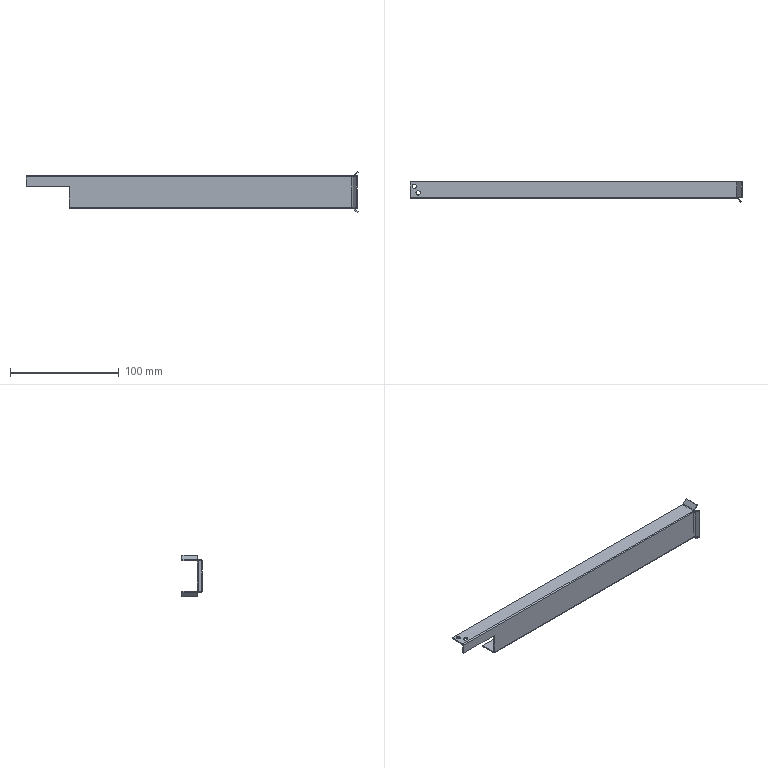Part | NX | 1 solid | 39 faces | box 305.707 x 18.464 x 38.21 mm | volume 16264 mm3 | plane 22 | cylinder 15 | torus 2 | commonest cylinder face diameters 4 x6 2 x4 6 x4 2.56 x1
STEP:
#1=CARTESIAN_POINT('',(150.133,-6.501,-15.));
#2=VERTEX_POINT('',#1);
#3=CARTESIAN_POINT('',(150.133,7.5,-15.));
#4=VERTEX_POINT('',#3);
#5=CARTESIAN_POINT('',(150.133,7.5,-15.));
#6=DIRECTION('',(0.,1.,0.));
#7=VECTOR('',#6,1000.);
#8=LINE('',#5,#7);
#9=EDGE_CURVE('',#2,#4,#8,.T.);
#10=ORIENTED_EDGE('',*,*,#9,.F.);
#11=CARTESIAN_POINT('',(150.,-6.5,-15.));
#12=VERTEX_POINT('',#11);
#13=CARTESIAN_POINT('',(150.,-9.5,-15.));
#14=DIRECTION('',(0.,0.,-1.));
#15=DIRECTION('',(0.,1.,0.));
#16=AXIS2_PLACEMENT_3D('',#13,#14,#15);
#17=CIRCLE('',#16,3.);
#18=EDGE_CURVE('',#12,#2,#17,.T.);
#19=ORIENTED_EDGE('',*,*,#18,.F.);
#20=CARTESIAN_POINT('',(-110.,-6.5,-15.));
#21=VERTEX_POINT('',#20);
#22=CARTESIAN_POINT('',(150.722,-6.5,-15.));
#23=DIRECTION('',(-1.,0.,0.));
#24=VECTOR('',#23,1000.);
#25=LINE('',#22,#24);
#26=EDGE_CURVE('',#12,#21,#25,.T.);
#27=ORIENTED_EDGE('',*,*,#26,.T.);
#28=CARTESIAN_POINT('',(-110.,7.5,-15.));
#29=VERTEX_POINT('',#28);
#30=CARTESIAN_POINT('',(-110.,7.5,-15.));
#31=DIRECTION('',(0.,-1.,0.));
#32=VECTOR('',#31,1000.);
#33=LINE('',#30,#32);
#34=EDGE_CURVE('',#29,#21,#33,.T.);
#35=ORIENTED_EDGE('',*,*,#34,.F.);
#36=CARTESIAN_POINT('',(-110.,7.5,-15.));
#37=DIRECTION('',(1.,0.,0.));
#38=VECTOR('',#37,1000.);
#39=LINE('',#36,#38);
#40=EDGE_CURVE('',#29,#4,#39,.T.);
#41=ORIENTED_EDGE('',*,*,#40,.T.);
#42=EDGE_LOOP('',(#10,#19,#27,#35,#41));
#43=FACE_BOUND('',#42,.T.);
#44=CARTESIAN_POINT('',(0.,0.,-15.));
#45=DIRECTION('',(0.,0.,1.));
#46=DIRECTION('',(1.,0.,0.));
#47=AXIS2_PLACEMENT_3D('',#44,#45,#46);
#48=PLANE('',#47);
#49=ADVANCED_FACE('',(#43),#48,.F.);
#50=CARTESIAN_POINT('',(151.547,7.5,-15.586));
#51=VERTEX_POINT('',#50);
#52=CARTESIAN_POINT('',(150.133,7.5,-17.));
#53=DIRECTION('',(0.,1.,0.));
#54=DIRECTION('',(0.,0.,1.));
#55=AXIS2_PLACEMENT_3D('',#52,#53,#54);
#56=CIRCLE('',#55,2.);
#57=EDGE_CURVE('',#4,#51,#56,.T.);
#58=ORIENTED_EDGE('',*,*,#57,.T.);
#59=CARTESIAN_POINT('',(151.547,-6.5,-15.586));
#60=VERTEX_POINT('',#59);
#61=CARTESIAN_POINT('',(151.547,-6.5,-15.586));
#62=DIRECTION('',(0.,1.,0.));
#63=VECTOR('',#62,1000.);
#64=LINE('',#61,#63);
#65=EDGE_CURVE('',#60,#51,#64,.T.);
#66=ORIENTED_EDGE('',*,*,#65,.F.);
#67=CARTESIAN_POINT('',(150.133,-6.5,-17.));
#68=DIRECTION('',(0.,-1.,0.));
#69=DIRECTION('',(0.7071,0.,0.7071));
#70=AXIS2_PLACEMENT_3D('',#67,#68,#69);
#71=CIRCLE('',#70,2.);
#72=EDGE_CURVE('',#60,#2,#71,.T.);
#73=ORIENTED_EDGE('',*,*,#72,.T.);
#74=ORIENTED_EDGE('',*,*,#9,.T.);
#75=EDGE_LOOP('',(#58,#66,#73,#74));
#76=FACE_BOUND('',#75,.T.);
#77=CARTESIAN_POINT('',(150.133,7.5,-17.));
#78=DIRECTION('',(0.,1.,0.));
#79=DIRECTION('',(0.,0.,1.));
#80=AXIS2_PLACEMENT_3D('',#77,#78,#79);
#81=CYLINDRICAL_SURFACE('',#80,2.);
#82=ADVANCED_FACE('',(#76),#81,.F.);
#83=ORIENTED_EDGE('',*,*,#40,.F.);
#84=CARTESIAN_POINT('',(-110.,7.5,-14.));
#85=VERTEX_POINT('',#84);
#86=CARTESIAN_POINT('',(-110.,7.5,-14.));
#87=DIRECTION('',(0.,0.,-1.));
#88=VECTOR('',#87,1000.);
#89=LINE('',#86,#88);
#90=EDGE_CURVE('',#85,#29,#89,.T.);
#91=ORIENTED_EDGE('',*,*,#90,.F.);
#92=CARTESIAN_POINT('',(149.99,7.5,-14.003));
#93=VERTEX_POINT('',#92);
#94=CARTESIAN_POINT('',(-110.,7.5,-14.));
#95=CARTESIAN_POINT('',(-23.337,7.5,-14.001));
#96=CARTESIAN_POINT('',(63.327,7.5,-14.002));
#97=CARTESIAN_POINT('',(149.99,7.5,-14.003));
#98=B_SPLINE_CURVE_WITH_KNOTS('',3,(#94,#95,#96,#97),.UNSPECIFIED.,.F.,.F.,(4,4),(0.,1.),.UNSPECIFIED.);
#99=EDGE_CURVE('',#93,#85,#98,.F.);
#100=ORIENTED_EDGE('',*,*,#99,.F.);
#101=CARTESIAN_POINT('',(150.133,7.5,-14.));
#102=VERTEX_POINT('',#101);
#103=CARTESIAN_POINT('',(150.133,7.5,-17.));
#104=DIRECTION('',(0.,-1.,0.));
#105=DIRECTION('',(0.000001761,0.,1.));
#106=AXIS2_PLACEMENT_3D('',#103,#104,#105);
#107=CIRCLE('',#106,3.);
#108=EDGE_CURVE('',#102,#93,#107,.T.);
#109=ORIENTED_EDGE('',*,*,#108,.F.);
#110=CARTESIAN_POINT('',(152.254,7.5,-14.878));
#111=VERTEX_POINT('',#110);
#112=CARTESIAN_POINT('',(150.133,7.5,-17.));
#113=DIRECTION('',(0.,-1.,0.));
#114=DIRECTION('',(0.000001761,0.,1.));
#115=AXIS2_PLACEMENT_3D('',#112,#113,#114);
#116=CIRCLE('',#115,3.);
#117=EDGE_CURVE('',#111,#102,#116,.T.);
#118=ORIENTED_EDGE('',*,*,#117,.F.);
#119=CARTESIAN_POINT('',(155.707,7.5,-18.331));
#120=VERTEX_POINT('',#119);
#121=CARTESIAN_POINT('',(155.707,7.5,-18.331));
#122=DIRECTION('',(-0.7071,0.,0.7071));
#123=VECTOR('',#122,1000.);
#124=LINE('',#121,#123);
#125=EDGE_CURVE('',#120,#111,#124,.T.);
#126=ORIENTED_EDGE('',*,*,#125,.F.);
#127=CARTESIAN_POINT('',(155.,7.5,-19.039));
#128=VERTEX_POINT('',#127);
#129=CARTESIAN_POINT('',(155.,7.5,-19.039));
#130=DIRECTION('',(0.7071,0.,0.7071));
#131=VECTOR('',#130,1000.);
#132=LINE('',#129,#131);
#133=EDGE_CURVE('',#128,#120,#132,.T.);
#134=ORIENTED_EDGE('',*,*,#133,.F.);
#135=CARTESIAN_POINT('',(151.547,7.5,-15.586));
#136=DIRECTION('',(0.7071,0.,-0.7071));
#137=VECTOR('',#136,1000.);
#138=LINE('',#135,#137);
#139=EDGE_CURVE('',#51,#128,#138,.T.);
#140=ORIENTED_EDGE('',*,*,#139,.F.);
#141=ORIENTED_EDGE('',*,*,#57,.F.);
#142=EDGE_LOOP('',(#83,#91,#100,#109,#118,#126,#134,#140,#141));
#143=FACE_BOUND('',#142,.T.);
#144=CARTESIAN_POINT('',(0.,7.5,-15.));
#145=DIRECTION('',(0.,1.,0.));
#146=DIRECTION('',(1.,0.,0.));
#147=AXIS2_PLACEMENT_3D('',#144,#145,#146);
#148=PLANE('',#147);
#149=ADVANCED_FACE('',(#143),#148,.T.);
#150=ORIENTED_EDGE('',*,*,#139,.T.);
#151=CARTESIAN_POINT('',(155.,-6.5,-19.039));
#152=VERTEX_POINT('',#151);
#153=CARTESIAN_POINT('',(155.,7.5,-19.039));
#154=DIRECTION('',(0.,-1.,0.));
#155=VECTOR('',#154,1000.);
#156=LINE('',#153,#155);
#157=EDGE_CURVE('',#128,#152,#156,.T.);
#158=ORIENTED_EDGE('',*,*,#157,.T.);
#159=CARTESIAN_POINT('',(155.,-6.5,-19.039));
#160=DIRECTION('',(-0.7071,0.,0.7071));
#161=VECTOR('',#160,1000.);
#162=LINE('',#159,#161);
#163=EDGE_CURVE('',#152,#60,#162,.T.);
#164=ORIENTED_EDGE('',*,*,#163,.T.);
#165=ORIENTED_EDGE('',*,*,#65,.T.);
#166=EDGE_LOOP('',(#150,#158,#164,#165));
#167=FACE_BOUND('',#166,.T.);
#168=CARTESIAN_POINT('',(155.,7.5,-19.039));
#169=DIRECTION('',(-0.7071,0.,-0.7071));
#170=DIRECTION('',(-0.7071,0.,0.7071));
#171=AXIS2_PLACEMENT_3D('',#168,#169,#170);
#172=PLANE('',#171);
#173=ADVANCED_FACE('',(#167),#172,.T.);
#174=CARTESIAN_POINT('',(150.,-6.5,-15.));
#175=VERTEX_POINT('',#174);
#176=CARTESIAN_POINT('',(150.,-6.5,-15.));
#177=CARTESIAN_POINT('',(150.044,-6.5,-15.));
#178=CARTESIAN_POINT('',(150.089,-6.5,-15.));
#179=CARTESIAN_POINT('',(150.133,-6.5,-15.));
#180=B_SPLINE_CURVE_WITH_KNOTS('',3,(#176,#177,#178,#179),.UNSPECIFIED.,.F.,.F.,(4,4),(0.,1.),.UNSPECIFIED.);
#181=EDGE_CURVE('',#175,#2,#180,.T.);
#182=ORIENTED_EDGE('',*,*,#181,.T.);
#183=ORIENTED_EDGE('',*,*,#72,.F.);
#184=ORIENTED_EDGE('',*,*,#163,.F.);
#185=CARTESIAN_POINT('',(155.707,-6.5,-18.331));
#186=VERTEX_POINT('',#185);
#187=CARTESIAN_POINT('',(155.707,-6.5,-18.331));
#188=DIRECTION('',(-0.7071,0.,-0.7071));
#189=VECTOR('',#188,1000.);
#190=LINE('',#187,#189);
#191=EDGE_CURVE('',#186,#152,#190,.T.);
#192=ORIENTED_EDGE('',*,*,#191,.F.);
#193=CARTESIAN_POINT('',(152.254,-6.5,-14.879));
#194=VERTEX_POINT('',#193);
#195=CARTESIAN_POINT('',(152.254,-6.5,-14.879));
#196=DIRECTION('',(0.7071,0.,-0.7071));
#197=VECTOR('',#196,1000.);
#198=LINE('',#195,#197);
#199=EDGE_CURVE('',#194,#186,#198,.T.);
#200=ORIENTED_EDGE('',*,*,#199,.F.);
#201=CARTESIAN_POINT('',(150.133,-6.5,-14.));
#202=VERTEX_POINT('',#201);
#203=CARTESIAN_POINT('',(150.133,-6.5,-17.));
#204=DIRECTION('',(0.,1.,0.));
#205=DIRECTION('',(0.,0.,1.));
#206=AXIS2_PLACEMENT_3D('',#203,#204,#205);
#207=CIRCLE('',#206,3.);
#208=EDGE_CURVE('',#202,#194,#207,.T.);
#209=ORIENTED_EDGE('',*,*,#208,.F.);
#210=CARTESIAN_POINT('',(150.,-6.5,-14.002));
#211=VERTEX_POINT('',#210);
#212=CARTESIAN_POINT('',(150.133,-6.5,-17.));
#213=DIRECTION('',(0.,1.,0.));
#214=DIRECTION('',(0.,0.,1.));
#215=AXIS2_PLACEMENT_3D('',#212,#213,#214);
#216=CIRCLE('',#215,3.);
#217=EDGE_CURVE('',#211,#202,#216,.T.);
#218=ORIENTED_EDGE('',*,*,#217,.F.);
#219=CARTESIAN_POINT('',(150.,-6.5,-15.));
#220=DIRECTION('',(0.,0.,1.));
#221=VECTOR('',#220,1000.);
#222=LINE('',#219,#221);
#223=EDGE_CURVE('',#175,#211,#222,.T.);
#224=ORIENTED_EDGE('',*,*,#223,.F.);
#225=EDGE_LOOP('',(#182,#183,#184,#192,#200,#209,#218,#224));
#226=FACE_BOUND('',#225,.T.);
#227=CARTESIAN_POINT('',(0.,-6.5,-15.));
#228=DIRECTION('',(0.,1.,0.));
#229=DIRECTION('',(1.,0.,0.));
#230=AXIS2_PLACEMENT_3D('',#227,#228,#229);
#231=PLANE('',#230);
#232=ADVANCED_FACE('',(#226),#231,.F.);
#233=CARTESIAN_POINT('',(150.,-6.5,15.));
#234=VERTEX_POINT('',#233);
#235=CARTESIAN_POINT('',(152.121,-7.379,15.));
#236=VERTEX_POINT('',#235);
#237=CARTESIAN_POINT('',(150.,-9.5,15.));
#238=DIRECTION('',(0.,0.,-1.));
#239=DIRECTION('',(0.,1.,0.));
#240=AXIS2_PLACEMENT_3D('',#237,#238,#239);
#241=CIRCLE('',#240,3.);
#242=EDGE_CURVE('',#234,#236,#241,.T.);
#243=ORIENTED_EDGE('',*,*,#242,.T.);
#244=CARTESIAN_POINT('',(152.121,-7.379,-15.));
#245=VERTEX_POINT('',#244);
#246=CARTESIAN_POINT('',(152.121,-7.379,-15.));
#247=DIRECTION('',(0.,0.,1.));
#248=VECTOR('',#247,1000.);
#249=LINE('',#246,#248);
#250=EDGE_CURVE('',#245,#236,#249,.T.);
#251=ORIENTED_EDGE('',*,*,#250,.F.);
#252=CARTESIAN_POINT('',(150.,-9.5,-15.));
#253=DIRECTION('',(0.,0.,1.));
#254=DIRECTION('',(0.7071,0.7071,0.));
#255=AXIS2_PLACEMENT_3D('',#252,#253,#254);
#256=CIRCLE('',#255,3.);
#257=EDGE_CURVE('',#245,#2,#256,.T.);
#258=ORIENTED_EDGE('',*,*,#257,.T.);
#259=ORIENTED_EDGE('',*,*,#181,.F.);
#260=ORIENTED_EDGE('',*,*,#223,.T.);
#261=CARTESIAN_POINT('',(150.,-6.5,14.));
#262=VERTEX_POINT('',#261);
#263=CARTESIAN_POINT('',(150.,-6.5,-15.));
#264=DIRECTION('',(0.,0.,1.));
#265=VECTOR('',#264,1000.);
#266=LINE('',#263,#265);
#267=EDGE_CURVE('',#211,#262,#266,.T.);
#268=ORIENTED_EDGE('',*,*,#267,.T.);
#269=CARTESIAN_POINT('',(150.,-6.5,-15.));
#270=DIRECTION('',(0.,0.,1.));
#271=VECTOR('',#270,1000.);
#272=LINE('',#269,#271);
#273=EDGE_CURVE('',#262,#234,#272,.T.);
#274=ORIENTED_EDGE('',*,*,#273,.T.);
#275=EDGE_LOOP('',(#243,#251,#258,#259,#260,#268,#274));
#276=FACE_BOUND('',#275,.T.);
#277=CARTESIAN_POINT('',(150.,-9.5,-15.));
#278=DIRECTION('',(0.,0.,1.));
#279=DIRECTION('',(0.,1.,0.));
#280=AXIS2_PLACEMENT_3D('',#277,#278,#279);
#281=CYLINDRICAL_SURFACE('',#280,3.);
#282=ADVANCED_FACE('',(#276),#281,.T.);
#283=CARTESIAN_POINT('',(151.414,-8.086,14.));
#284=VERTEX_POINT('',#283);
#285=CARTESIAN_POINT('',(150.,-7.5,14.));
#286=VERTEX_POINT('',#285);
#287=CARTESIAN_POINT('',(150.,-9.5,14.));
#288=DIRECTION('',(0.,0.,1.));
#289=DIRECTION('',(1.,0.,0.));
#290=AXIS2_PLACEMENT_3D('',#287,#288,#289);
#291=CIRCLE('',#290,2.);
#292=EDGE_CURVE('',#284,#286,#291,.T.);
#293=ORIENTED_EDGE('',*,*,#292,.F.);
#294=CARTESIAN_POINT('',(152.121,-7.379,14.));
#295=DIRECTION('',(0.7071,-0.7071,0.));
#296=DIRECTION('',(0.,0.,1.));
#297=AXIS2_PLACEMENT_3D('',#294,#295,#296);
#298=CIRCLE('',#297,1.);
#299=EDGE_CURVE('',#236,#284,#298,.T.);
#300=ORIENTED_EDGE('',*,*,#299,.F.);
#301=ORIENTED_EDGE('',*,*,#242,.F.);
#302=CARTESIAN_POINT('',(150.,-6.5,14.));
#303=DIRECTION('',(-1.,0.,0.));
#304=DIRECTION('',(0.,-1.,0.));
#305=AXIS2_PLACEMENT_3D('',#302,#303,#304);
#306=CIRCLE('',#305,1.);
#307=EDGE_CURVE('',#286,#234,#306,.T.);
#308=ORIENTED_EDGE('',*,*,#307,.F.);
#309=EDGE_LOOP('',(#293,#300,#301,#308));
#310=FACE_BOUND('',#309,.T.);
#311=CARTESIAN_POINT('',(150.,-9.5,14.));
#312=DIRECTION('',(0.,0.,1.));
#313=DIRECTION('',(1.,0.,0.));
#314=AXIS2_PLACEMENT_3D('',#311,#312,#313);
#315=TOROIDAL_SURFACE('',#314,3.,1.);
#316=ADVANCED_FACE('',(#310),#315,.T.);
#317=CARTESIAN_POINT('',(151.414,-8.086,-14.));
#318=VERTEX_POINT('',#317);
#319=CARTESIAN_POINT('',(150.,-7.5,-14.));
#320=VERTEX_POINT('',#319);
#321=CARTESIAN_POINT('',(150.,-9.5,-14.));
#322=DIRECTION('',(0.,0.,1.));
#323=DIRECTION('',(1.,0.,0.));
#324=AXIS2_PLACEMENT_3D('',#321,#322,#323);
#325=CIRCLE('',#324,2.);
#326=EDGE_CURVE('',#318,#320,#325,.T.);
#327=ORIENTED_EDGE('',*,*,#326,.F.);
#328=CARTESIAN_POINT('',(151.414,-8.086,14.));
#329=DIRECTION('',(0.,0.,-1.));
#330=VECTOR('',#329,1000.);
#331=LINE('',#328,#330);
#332=EDGE_CURVE('',#284,#318,#331,.T.);
#333=ORIENTED_EDGE('',*,*,#332,.F.);
#334=ORIENTED_EDGE('',*,*,#292,.T.);
#335=CARTESIAN_POINT('',(150.,-7.5,-15.));
#336=DIRECTION('',(0.,0.,1.));
#337=VECTOR('',#336,1000.);
#338=LINE('',#335,#337);
#339=EDGE_CURVE('',#320,#286,#338,.T.);
#340=ORIENTED_EDGE('',*,*,#339,.F.);
#341=EDGE_LOOP('',(#327,#333,#334,#340));
#342=FACE_BOUND('',#341,.T.);
#343=CARTESIAN_POINT('',(150.,-9.5,-15.));
#344=DIRECTION('',(0.,0.,1.));
#345=DIRECTION('',(0.,1.,0.));
#346=AXIS2_PLACEMENT_3D('',#343,#344,#345);
#347=CYLINDRICAL_SURFACE('',#346,2.);
#348=ADVANCED_FACE('',(#342),#347,.F.);
#349=ORIENTED_EDGE('',*,*,#257,.F.);
#350=CARTESIAN_POINT('',(152.121,-7.379,-14.));
#351=DIRECTION('',(0.7071,-0.7071,0.));
#352=DIRECTION('',(-0.7071,-0.7071,0.));
#353=AXIS2_PLACEMENT_3D('',#350,#351,#352);
#354=CIRCLE('',#353,1.);
#355=EDGE_CURVE('',#318,#245,#354,.T.);
#356=ORIENTED_EDGE('',*,*,#355,.F.);
#357=ORIENTED_EDGE('',*,*,#326,.T.);
#358=CARTESIAN_POINT('',(150.,-6.5,-14.));
#359=DIRECTION('',(-1.,0.,0.));
#360=DIRECTION('',(0.,0.,-1.));
#361=AXIS2_PLACEMENT_3D('',#358,#359,#360);
#362=CIRCLE('',#361,1.);
#363=EDGE_CURVE('',#12,#320,#362,.T.);
#364=ORIENTED_EDGE('',*,*,#363,.F.);
#365=ORIENTED_EDGE('',*,*,#18,.T.);
#366=EDGE_LOOP('',(#349,#356,#357,#364,#365));
#367=FACE_BOUND('',#366,.T.);
#368=CARTESIAN_POINT('',(150.,-9.5,-14.));
#369=DIRECTION('',(0.,0.,1.));
#370=DIRECTION('',(1.,0.,0.));
#371=AXIS2_PLACEMENT_3D('',#368,#369,#370);
#372=TOROIDAL_SURFACE('',#371,3.,1.);
#373=ADVANCED_FACE('',(#367),#372,.T.);
#374=CARTESIAN_POINT('',(-110.,-7.5,-14.));
#375=VERTEX_POINT('',#374);
#376=CARTESIAN_POINT('',(-110.,-7.5,-14.));
#377=DIRECTION('',(1.,0.,0.));
#378=VECTOR('',#377,1000.);
#379=LINE('',#376,#378);
#380=EDGE_CURVE('',#375,#320,#379,.T.);
#381=ORIENTED_EDGE('',*,*,#380,.F.);
#382=CARTESIAN_POINT('',(-110.,-6.5,-14.));
#383=DIRECTION('',(1.,0.,0.));
#384=DIRECTION('',(0.,-1.,0.));
#385=AXIS2_PLACEMENT_3D('',#382,#383,#384);
#386=CIRCLE('',#385,1.);
#387=EDGE_CURVE('',#375,#21,#386,.T.);
#388=ORIENTED_EDGE('',*,*,#387,.T.);
#389=ORIENTED_EDGE('',*,*,#26,.F.);
#390=ORIENTED_EDGE('',*,*,#363,.T.);
#391=EDGE_LOOP('',(#381,#388,#389,#390));
#392=FACE_BOUND('',#391,.T.);
#393=CARTESIAN_POINT('',(150.722,-6.5,-14.));
#394=DIRECTION('',(-1.,0.,0.));
#395=DIRECTION('',(0.,0.,-1.));
#396=AXIS2_PLACEMENT_3D('',#393,#394,#395);
#397=CYLINDRICAL_SURFACE('',#396,1.);
#398=ADVANCED_FACE('',(#392),#397,.T.);
#399=ORIENTED_EDGE('',*,*,#380,.T.);
#400=ORIENTED_EDGE('',*,*,#339,.T.);
#401=CARTESIAN_POINT('',(-150.,-7.5,14.));
#402=VERTEX_POINT('',#401);
#403=CARTESIAN_POINT('',(150.,-7.5,14.));
#404=DIRECTION('',(-1.,0.,0.));
#405=VECTOR('',#404,1000.);
#406=LINE('',#403,#405);
#407=EDGE_CURVE('',#286,#402,#406,.T.);
#408=ORIENTED_EDGE('',*,*,#407,.T.);
#409=CARTESIAN_POINT('',(-150.,-7.5,5.));
#410=VERTEX_POINT('',#409);
#411=CARTESIAN_POINT('',(-150.,-7.5,14.));
#412=DIRECTION('',(0.,0.,-1.));
#413=VECTOR('',#412,1000.);
#414=LINE('',#411,#413);
#415=EDGE_CURVE('',#402,#410,#414,.T.);
#416=ORIENTED_EDGE('',*,*,#415,.T.);
#417=CARTESIAN_POINT('',(-110.,-7.5,5.));
#418=VERTEX_POINT('',#417);
#419=CARTESIAN_POINT('',(-110.,-7.5,5.));
#420=DIRECTION('',(-1.,0.,0.));
#421=VECTOR('',#420,1000.);
#422=LINE('',#419,#421);
#423=EDGE_CURVE('',#418,#410,#422,.T.);
#424=ORIENTED_EDGE('',*,*,#423,.F.);
#425=CARTESIAN_POINT('',(-110.,-7.5,5.));
#426=DIRECTION('',(0.,0.,-1.));
#427=VECTOR('',#426,1000.);
#428=LINE('',#425,#427);
#429=EDGE_CURVE('',#418,#375,#428,.T.);
#430=ORIENTED_EDGE('',*,*,#429,.T.);
#431=EDGE_LOOP('',(#399,#400,#408,#416,#424,#430));
#432=FACE_BOUND('',#431,.T.);
#433=CARTESIAN_POINT('',(-150.,-7.5,-15.));
#434=DIRECTION('',(0.,-1.,0.));
#435=DIRECTION('',(0.,0.,-1.));
#436=AXIS2_PLACEMENT_3D('',#433,#434,#435);
#437=PLANE('',#436);
#438=ADVANCED_FACE('',(#432),#437,.T.);
#439=ORIENTED_EDGE('',*,*,#387,.F.);
#440=ORIENTED_EDGE('',*,*,#429,.F.);
#441=CARTESIAN_POINT('',(-110.,-6.5,5.));
#442=VERTEX_POINT('',#441);
#443=CARTESIAN_POINT('',(-110.,-6.5,5.));
#444=DIRECTION('',(0.,-1.,0.));
#445=VECTOR('',#444,1000.);
#446=LINE('',#443,#445);
#447=EDGE_CURVE('',#442,#418,#446,.T.);
#448=ORIENTED_EDGE('',*,*,#447,.F.);
#449=CARTESIAN_POINT('',(-110.,-6.5,-14.));
#450=VERTEX_POINT('',#449);
#451=CARTESIAN_POINT('',(-110.,-6.5,5.));
#452=DIRECTION('',(0.,0.,-1.));
#453=VECTOR('',#452,1000.);
#454=LINE('',#451,#453);
#455=EDGE_CURVE('',#442,#450,#454,.T.);
#456=ORIENTED_EDGE('',*,*,#455,.T.);
#457=CARTESIAN_POINT('',(-110.,-6.5,-14.));
#458=CARTESIAN_POINT('',(-110.,-1.833,-14.));
#459=CARTESIAN_POINT('',(-110.,2.833,-14.));
#460=CARTESIAN_POINT('',(-110.,7.5,-14.));
#461=B_SPLINE_CURVE_WITH_KNOTS('',3,(#457,#458,#459,#460),.UNSPECIFIED.,.F.,.F.,(4,4),(0.,1.),.UNSPECIFIED.);
#462=EDGE_CURVE('',#85,#450,#461,.F.);
#463=ORIENTED_EDGE('',*,*,#462,.F.);
#464=ORIENTED_EDGE('',*,*,#90,.T.);
#465=ORIENTED_EDGE('',*,*,#34,.T.);
#466=EDGE_LOOP('',(#439,#440,#448,#456,#463,#464,#465));
#467=FACE_BOUND('',#466,.T.);
#468=CARTESIAN_POINT('',(-110.,-7.5,-15.));
#469=DIRECTION('',(1.,0.,0.));
#470=DIRECTION('',(0.,1.,0.));
#471=AXIS2_PLACEMENT_3D('',#468,#469,#470);
#472=PLANE('',#471);
#473=ADVANCED_FACE('',(#467),#472,.F.);
#474=ORIENTED_EDGE('',*,*,#99,.T.);
#475=ORIENTED_EDGE('',*,*,#462,.T.);
#476=CARTESIAN_POINT('',(-110.,-6.5,-14.));
#477=CARTESIAN_POINT('',(-23.333,-6.5,-14.));
#478=CARTESIAN_POINT('',(63.333,-6.5,-14.));
#479=CARTESIAN_POINT('',(150.,-6.5,-14.));
#480=B_SPLINE_CURVE_WITH_KNOTS('',3,(#476,#477,#478,#479),.UNSPECIFIED.,.F.,.F.,(4,4),(0.,1.),.UNSPECIFIED.);
#481=EDGE_CURVE('',#450,#211,#480,.T.);
#482=ORIENTED_EDGE('',*,*,#481,.T.);
#483=CARTESIAN_POINT('',(150.,-6.5,-14.));
#484=CARTESIAN_POINT('',(149.997,-1.833,-14.));
#485=CARTESIAN_POINT('',(149.993,2.833,-14.));
#486=CARTESIAN_POINT('',(149.99,7.5,-14.));
#487=B_SPLINE_CURVE_WITH_KNOTS('',3,(#483,#484,#485,#486),.UNSPECIFIED.,.F.,.F.,(4,4),(0.,1.),.UNSPECIFIED.);
#488=EDGE_CURVE('',#93,#211,#487,.F.);
#489=ORIENTED_EDGE('',*,*,#488,.F.);
#490=EDGE_LOOP('',(#474,#475,#482,#489));
#491=FACE_BOUND('',#490,.T.);
#492=CARTESIAN_POINT('',(0.,-6.5,-14.));
#493=DIRECTION('',(0.,0.,1.));
#494=DIRECTION('',(1.,0.,0.));
#495=AXIS2_PLACEMENT_3D('',#492,#493,#494);
#496=PLANE('',#495);
#497=ADVANCED_FACE('',(#491),#496,.T.);
#498=CARTESIAN_POINT('',(150.133,7.5,-14.));
#499=DIRECTION('',(0.,1.,0.));
#500=VECTOR('',#499,1000.);
#501=LINE('',#498,#500);
#502=EDGE_CURVE('',#202,#102,#501,.T.);
#503=ORIENTED_EDGE('',*,*,#502,.F.);
#504=ORIENTED_EDGE('',*,*,#208,.T.);
#505=CARTESIAN_POINT('',(152.254,7.5,-14.878));
#506=DIRECTION('',(0.00001609,-1.,-0.00001609));
#507=VECTOR('',#506,1000.);
#508=LINE('',#505,#507);
#509=EDGE_CURVE('',#111,#194,#508,.T.);
#510=ORIENTED_EDGE('',*,*,#509,.F.);
#511=ORIENTED_EDGE('',*,*,#117,.T.);
#512=EDGE_LOOP('',(#503,#504,#510,#511));
#513=FACE_BOUND('',#512,.T.);
#514=CARTESIAN_POINT('',(150.133,7.5,-17.));
#515=DIRECTION('',(0.,1.,0.));
#516=DIRECTION('',(0.,0.,1.));
#517=AXIS2_PLACEMENT_3D('',#514,#515,#516);
#518=CYLINDRICAL_SURFACE('',#517,3.);
#519=ADVANCED_FACE('',(#513),#518,.T.);
#520=ORIENTED_EDGE('',*,*,#125,.T.);
#521=ORIENTED_EDGE('',*,*,#509,.T.);
#522=ORIENTED_EDGE('',*,*,#199,.T.);
#523=CARTESIAN_POINT('',(155.707,7.5,-18.331));
#524=DIRECTION('',(0.,-1.,0.));
#525=VECTOR('',#524,1000.);
#526=LINE('',#523,#525);
#527=EDGE_CURVE('',#120,#186,#526,.T.);
#528=ORIENTED_EDGE('',*,*,#527,.F.);
#529=EDGE_LOOP('',(#520,#521,#522,#528));
#530=FACE_BOUND('',#529,.T.);
#531=CARTESIAN_POINT('',(152.254,7.5,-14.879));
#532=DIRECTION('',(0.7071,0.,0.7071));
#533=DIRECTION('',(0.,-1.,0.));
#534=AXIS2_PLACEMENT_3D('',#531,#532,#533);
#535=PLANE('',#534);
#536=ADVANCED_FACE('',(#530),#535,.T.);
#537=ORIENTED_EDGE('',*,*,#133,.T.);
#538=ORIENTED_EDGE('',*,*,#527,.T.);
#539=ORIENTED_EDGE('',*,*,#191,.T.);
#540=ORIENTED_EDGE('',*,*,#157,.F.);
#541=EDGE_LOOP('',(#537,#538,#539,#540));
#542=FACE_BOUND('',#541,.T.);
#543=CARTESIAN_POINT('',(155.707,7.5,-18.331));
#544=DIRECTION('',(0.7071,0.,-0.7071));
#545=DIRECTION('',(0.,-1.,0.));
#546=AXIS2_PLACEMENT_3D('',#543,#544,#545);
#547=PLANE('',#546);
#548=ADVANCED_FACE('',(#542),#547,.T.);
#549=ORIENTED_EDGE('',*,*,#481,.F.);
#550=ORIENTED_EDGE('',*,*,#455,.F.);
#551=CARTESIAN_POINT('',(-150.,-6.5,5.));
#552=VERTEX_POINT('',#551);
#553=CARTESIAN_POINT('',(-110.,-6.5,5.));
#554=DIRECTION('',(-1.,0.,0.));
#555=VECTOR('',#554,1000.);
#556=LINE('',#553,#555);
#557=EDGE_CURVE('',#442,#552,#556,.T.);
#558=ORIENTED_EDGE('',*,*,#557,.T.);
#559=CARTESIAN_POINT('',(-150.,-6.5,14.));
#560=VERTEX_POINT('',#559);
#561=CARTESIAN_POINT('',(-150.,-6.5,14.));
#562=DIRECTION('',(0.,0.,-1.));
#563=VECTOR('',#562,1000.);
#564=LINE('',#561,#563);
#565=EDGE_CURVE('',#560,#552,#564,.T.);
#566=ORIENTED_EDGE('',*,*,#565,.F.);
#567=CARTESIAN_POINT('',(150.,-6.5,14.));
#568=DIRECTION('',(-1.,0.,0.));
#569=VECTOR('',#568,1000.);
#570=LINE('',#567,#569);
#571=EDGE_CURVE('',#262,#560,#570,.T.);
#572=ORIENTED_EDGE('',*,*,#571,.F.);
#573=ORIENTED_EDGE('',*,*,#267,.F.);
#574=EDGE_LOOP('',(#549,#550,#558,#566,#572,#573));
#575=FACE_BOUND('',#574,.T.);
#576=CARTESIAN_POINT('',(-150.,-6.5,-15.));
#577=DIRECTION('',(0.,-1.,0.));
#578=DIRECTION('',(0.,0.,-1.));
#579=AXIS2_PLACEMENT_3D('',#576,#577,#578);
#580=PLANE('',#579);
#581=ADVANCED_FACE('',(#575),#580,.F.);
#582=CARTESIAN_POINT('',(-150.,7.5,14.));
#583=VERTEX_POINT('',#582);
#584=CARTESIAN_POINT('',(150.,7.5,14.));
#585=VERTEX_POINT('',#584);
#586=CARTESIAN_POINT('',(-150.,7.5,14.));
#587=DIRECTION('',(1.,0.,0.));
#588=VECTOR('',#587,1000.);
#589=LINE('',#586,#588);
#590=EDGE_CURVE('',#583,#585,#589,.T.);
#591=ORIENTED_EDGE('',*,*,#590,.T.);
#592=CARTESIAN_POINT('',(150.,7.5,14.));
#593=DIRECTION('',(0.,-1.,0.));
#594=VECTOR('',#593,1000.);
#595=LINE('',#592,#594);
#596=EDGE_CURVE('',#585,#262,#595,.T.);
#597=ORIENTED_EDGE('',*,*,#596,.T.);
#598=ORIENTED_EDGE('',*,*,#571,.T.);
#599=CARTESIAN_POINT('',(-150.,7.5,14.));
#600=DIRECTION('',(0.,-1.,0.));
#601=VECTOR('',#600,1000.);
#602=LINE('',#599,#601);
#603=EDGE_CURVE('',#583,#560,#602,.T.);
#604=ORIENTED_EDGE('',*,*,#603,.F.);
#605=EDGE_LOOP('',(#591,#597,#598,#604));
#606=FACE_BOUND('',#605,.T.);
#607=CARTESIAN_POINT('',(-148.,3.5,14.));
#608=VERTEX_POINT('',#607);
#609=CARTESIAN_POINT('',(-144.,3.5,14.));
#610=VERTEX_POINT('',#609);
#611=CARTESIAN_POINT('',(-146.,3.5,14.));
#612=DIRECTION('',(0.,0.,-1.));
#613=DIRECTION('',(-1.,0.,0.));
#614=AXIS2_PLACEMENT_3D('',#611,#612,#613);
#615=CIRCLE('',#614,2.);
#616=EDGE_CURVE('',#608,#610,#615,.T.);
#617=ORIENTED_EDGE('',*,*,#616,.F.);
#618=CARTESIAN_POINT('',(-146.,3.5,14.));
#619=DIRECTION('',(0.,0.,-1.));
#620=DIRECTION('',(-1.,0.,0.));
#621=AXIS2_PLACEMENT_3D('',#618,#619,#620);
#622=CIRCLE('',#621,2.);
#623=EDGE_CURVE('',#610,#608,#622,.T.);
#624=ORIENTED_EDGE('',*,*,#623,.F.);
#625=EDGE_LOOP('',(#617,#624));
#626=FACE_BOUND('',#625,.T.);
#627=CARTESIAN_POINT('',(-140.5,-2.562,14.));
#628=VERTEX_POINT('',#627);
#629=CARTESIAN_POINT('',(-144.5,-2.562,14.));
#630=VERTEX_POINT('',#629);
#631=CARTESIAN_POINT('',(-142.5,-2.562,14.));
#632=DIRECTION('',(0.,0.,-1.));
#633=DIRECTION('',(-1.,0.,0.));
#634=AXIS2_PLACEMENT_3D('',#631,#632,#633);
#635=CIRCLE('',#634,2.);
#636=EDGE_CURVE('',#628,#630,#635,.T.);
#637=ORIENTED_EDGE('',*,*,#636,.F.);
#638=CARTESIAN_POINT('',(-142.5,-2.562,14.));
#639=DIRECTION('',(0.,0.,-1.));
#640=DIRECTION('',(-1.,0.,0.));
#641=AXIS2_PLACEMENT_3D('',#638,#639,#640);
#642=CIRCLE('',#641,2.);
#643=EDGE_CURVE('',#630,#628,#642,.T.);
#644=ORIENTED_EDGE('',*,*,#643,.F.);
#645=EDGE_LOOP('',(#637,#644));
#646=FACE_BOUND('',#645,.T.);
#647=CARTESIAN_POINT('',(0.,0.,14.));
#648=DIRECTION('',(0.,0.,1.));
#649=DIRECTION('',(1.,0.,0.));
#650=AXIS2_PLACEMENT_3D('',#647,#648,#649);
#651=PLANE('',#650);
#652=ADVANCED_FACE('',(#606,#626,#646),#651,.F.);
#653=ORIENTED_EDGE('',*,*,#590,.F.);
#654=CARTESIAN_POINT('',(-150.,7.5,15.));
#655=VERTEX_POINT('',#654);
#656=CARTESIAN_POINT('',(-150.,7.5,15.));
#657=DIRECTION('',(0.,0.,-1.));
#658=VECTOR('',#657,1000.);
#659=LINE('',#656,#658);
#660=EDGE_CURVE('',#655,#583,#659,.T.);
#661=ORIENTED_EDGE('',*,*,#660,.F.);
#662=CARTESIAN_POINT('',(150.298,7.5,15.));
#663=VERTEX_POINT('',#662);
#664=CARTESIAN_POINT('',(150.298,7.5,15.));
#665=DIRECTION('',(-1.,0.,0.));
#666=VECTOR('',#665,1000.);
#667=LINE('',#664,#666);
#668=EDGE_CURVE('',#663,#655,#667,.T.);
#669=ORIENTED_EDGE('',*,*,#668,.F.);
#670=CARTESIAN_POINT('',(151.203,7.5,15.375));
#671=VERTEX_POINT('',#670);
#672=CARTESIAN_POINT('',(150.298,7.5,16.28));
#673=DIRECTION('',(0.,1.,0.));
#674=DIRECTION('',(0.7071,0.,-0.7071));
#675=AXIS2_PLACEMENT_3D('',#672,#673,#674);
#676=CIRCLE('',#675,1.28);
#677=EDGE_CURVE('',#671,#663,#676,.T.);
#678=ORIENTED_EDGE('',*,*,#677,.F.);
#679=CARTESIAN_POINT('',(155.,7.5,19.172));
#680=VERTEX_POINT('',#679);
#681=CARTESIAN_POINT('',(155.,7.5,19.172));
#682=DIRECTION('',(-0.7071,0.,-0.7071));
#683=VECTOR('',#682,1000.);
#684=LINE('',#681,#683);
#685=EDGE_CURVE('',#680,#671,#684,.T.);
#686=ORIENTED_EDGE('',*,*,#685,.F.);
#687=CARTESIAN_POINT('',(155.707,7.5,18.464));
#688=VERTEX_POINT('',#687);
#689=CARTESIAN_POINT('',(155.707,7.5,18.464));
#690=DIRECTION('',(-0.7071,0.,0.7071));
#691=VECTOR('',#690,1000.);
#692=LINE('',#689,#691);
#693=EDGE_CURVE('',#688,#680,#692,.T.);
#694=ORIENTED_EDGE('',*,*,#693,.F.);
#695=CARTESIAN_POINT('',(152.121,7.5,14.879));
#696=VERTEX_POINT('',#695);
#697=CARTESIAN_POINT('',(152.121,7.5,14.879));
#698=DIRECTION('',(0.7071,0.,0.7071));
#699=VECTOR('',#698,1000.);
#700=LINE('',#697,#699);
#701=EDGE_CURVE('',#696,#688,#700,.T.);
#702=ORIENTED_EDGE('',*,*,#701,.F.);
#703=CARTESIAN_POINT('',(150.,7.5,17.));
#704=DIRECTION('',(0.,-1.,0.));
#705=DIRECTION('',(0.,0.,-1.));
#706=AXIS2_PLACEMENT_3D('',#703,#704,#705);
#707=CIRCLE('',#706,3.);
#708=EDGE_CURVE('',#585,#696,#707,.T.);
#709=ORIENTED_EDGE('',*,*,#708,.F.);
#710=EDGE_LOOP('',(#653,#661,#669,#678,#686,#694,#702,#709));
#711=FACE_BOUND('',#710,.T.);
#712=CARTESIAN_POINT('',(150.,7.5,-15.));
#713=DIRECTION('',(0.,1.,0.));
#714=DIRECTION('',(1.,0.,0.));
#715=AXIS2_PLACEMENT_3D('',#712,#713,#714);
#716=PLANE('',#715);
#717=ADVANCED_FACE('',(#711),#716,.T.);
#718=ORIENTED_EDGE('',*,*,#708,.T.);
#719=CARTESIAN_POINT('',(152.121,-6.5,14.879));
#720=VERTEX_POINT('',#719);
#721=CARTESIAN_POINT('',(152.121,-6.5,14.879));
#722=DIRECTION('',(0.,1.,0.));
#723=VECTOR('',#722,1000.);
#724=LINE('',#721,#723);
#725=EDGE_CURVE('',#720,#696,#724,.T.);
#726=ORIENTED_EDGE('',*,*,#725,.F.);
#727=CARTESIAN_POINT('',(150.,-6.5,17.));
#728=DIRECTION('',(0.,1.,0.));
#729=DIRECTION('',(0.7071,0.,-0.7071));
#730=AXIS2_PLACEMENT_3D('',#727,#728,#729);
#731=CIRCLE('',#730,3.);
#732=EDGE_CURVE('',#720,#262,#731,.T.);
#733=ORIENTED_EDGE('',*,*,#732,.T.);
#734=ORIENTED_EDGE('',*,*,#596,.F.);
#735=EDGE_LOOP('',(#718,#726,#733,#734));
#736=FACE_BOUND('',#735,.T.);
#737=CARTESIAN_POINT('',(150.,7.5,17.));
#738=DIRECTION('',(0.,-1.,0.));
#739=DIRECTION('',(0.,0.,1.));
#740=AXIS2_PLACEMENT_3D('',#737,#738,#739);
#741=CYLINDRICAL_SURFACE('',#740,3.);
#742=ADVANCED_FACE('',(#736),#741,.T.);
#743=CARTESIAN_POINT('',(150.298,-6.5,15.));
#744=VERTEX_POINT('',#743);
#745=CARTESIAN_POINT('',(150.,-6.5,15.));
#746=DIRECTION('',(1.,0.,0.));
#747=VECTOR('',#746,1000.);
#748=LINE('',#745,#747);
#749=EDGE_CURVE('',#234,#744,#748,.T.);
#750=ORIENTED_EDGE('',*,*,#749,.F.);
#751=ORIENTED_EDGE('',*,*,#273,.F.);
#752=ORIENTED_EDGE('',*,*,#732,.F.);
#753=CARTESIAN_POINT('',(155.707,-6.5,18.464));
#754=VERTEX_POINT('',#753);
#755=CARTESIAN_POINT('',(155.707,-6.5,18.464));
#756=DIRECTION('',(-0.7071,0.,-0.7071));
#757=VECTOR('',#756,1000.);
#758=LINE('',#755,#757);
#759=EDGE_CURVE('',#754,#720,#758,.T.);
#760=ORIENTED_EDGE('',*,*,#759,.F.);
#761=CARTESIAN_POINT('',(155.,-6.5,19.172));
#762=VERTEX_POINT('',#761);
#763=CARTESIAN_POINT('',(155.,-6.5,19.172));
#764=DIRECTION('',(0.7071,0.,-0.7071));
#765=VECTOR('',#764,1000.);
#766=LINE('',#763,#765);
#767=EDGE_CURVE('',#762,#754,#766,.T.);
#768=ORIENTED_EDGE('',*,*,#767,.F.);
#769=CARTESIAN_POINT('',(151.203,-6.5,15.375));
#770=VERTEX_POINT('',#769);
#771=CARTESIAN_POINT('',(151.203,-6.5,15.375));
#772=DIRECTION('',(0.7071,0.,0.7071));
#773=VECTOR('',#772,1000.);
#774=LINE('',#771,#773);
#775=EDGE_CURVE('',#770,#762,#774,.T.);
#776=ORIENTED_EDGE('',*,*,#775,.F.);
#777=CARTESIAN_POINT('',(150.298,-6.5,16.28));
#778=DIRECTION('',(0.,-1.,0.));
#779=DIRECTION('',(0.,0.,-1.));
#780=AXIS2_PLACEMENT_3D('',#777,#778,#779);
#781=CIRCLE('',#780,1.28);
#782=EDGE_CURVE('',#744,#770,#781,.T.);
#783=ORIENTED_EDGE('',*,*,#782,.F.);
#784=EDGE_LOOP('',(#750,#751,#752,#760,#768,#776,#783));
#785=FACE_BOUND('',#784,.T.);
#786=CARTESIAN_POINT('',(0.,-6.5,-15.));
#787=DIRECTION('',(0.,-1.,0.));
#788=DIRECTION('',(0.,0.,-1.));
#789=AXIS2_PLACEMENT_3D('',#786,#787,#788);
#790=PLANE('',#789);
#791=ADVANCED_FACE('',(#785),#790,.T.);
#792=CARTESIAN_POINT('',(-150.,-6.5,15.));
#793=VERTEX_POINT('',#792);
#794=CARTESIAN_POINT('',(-150.508,-6.5,15.));
#795=DIRECTION('',(1.,0.,0.));
#796=VECTOR('',#795,1000.);
#797=LINE('',#794,#796);
#798=EDGE_CURVE('',#793,#234,#797,.T.);
#799=ORIENTED_EDGE('',*,*,#798,.T.);
#800=ORIENTED_EDGE('',*,*,#749,.T.);
#801=CARTESIAN_POINT('',(150.298,7.5,15.));
#802=DIRECTION('',(0.,-1.,0.));
#803=VECTOR('',#802,1000.);
#804=LINE('',#801,#803);
#805=EDGE_CURVE('',#663,#744,#804,.T.);
#806=ORIENTED_EDGE('',*,*,#805,.F.);
#807=ORIENTED_EDGE('',*,*,#668,.T.);
#808=CARTESIAN_POINT('',(-150.,-6.5,15.));
#809=DIRECTION('',(0.,1.,0.));
#810=VECTOR('',#809,1000.);
#811=LINE('',#808,#810);
#812=EDGE_CURVE('',#793,#655,#811,.T.);
#813=ORIENTED_EDGE('',*,*,#812,.F.);
#814=EDGE_LOOP('',(#799,#800,#806,#807,#813));
#815=FACE_BOUND('',#814,.T.);
#816=CARTESIAN_POINT('',(-148.,3.5,15.));
#817=VERTEX_POINT('',#816);
#818=CARTESIAN_POINT('',(-144.,3.5,15.));
#819=VERTEX_POINT('',#818);
#820=CARTESIAN_POINT('',(-146.,3.5,15.));
#821=DIRECTION('',(0.,0.,1.));
#822=DIRECTION('',(1.,0.,0.));
#823=AXIS2_PLACEMENT_3D('',#820,#821,#822);
#824=CIRCLE('',#823,2.);
#825=EDGE_CURVE('',#817,#819,#824,.T.);
#826=ORIENTED_EDGE('',*,*,#825,.F.);
#827=CARTESIAN_POINT('',(-146.,3.5,15.));
#828=DIRECTION('',(0.,0.,1.));
#829=DIRECTION('',(1.,0.,0.));
#830=AXIS2_PLACEMENT_3D('',#827,#828,#829);
#831=CIRCLE('',#830,2.);
#832=EDGE_CURVE('',#819,#817,#831,.T.);
#833=ORIENTED_EDGE('',*,*,#832,.F.);
#834=EDGE_LOOP('',(#826,#833));
#835=FACE_BOUND('',#834,.T.);
#836=CARTESIAN_POINT('',(-144.5,-2.562,15.));
#837=VERTEX_POINT('',#836);
#838=CARTESIAN_POINT('',(-140.5,-2.562,15.));
#839=VERTEX_POINT('',#838);
#840=CARTESIAN_POINT('',(-142.5,-2.562,15.));
#841=DIRECTION('',(0.,0.,1.));
#842=DIRECTION('',(1.,0.,0.));
#843=AXIS2_PLACEMENT_3D('',#840,#841,#842);
#844=CIRCLE('',#843,2.);
#845=EDGE_CURVE('',#837,#839,#844,.T.);
#846=ORIENTED_EDGE('',*,*,#845,.F.);
#847=CARTESIAN_POINT('',(-142.5,-2.562,15.));
#848=DIRECTION('',(0.,0.,1.));
#849=DIRECTION('',(1.,0.,0.));
#850=AXIS2_PLACEMENT_3D('',#847,#848,#849);
#851=CIRCLE('',#850,2.);
#852=EDGE_CURVE('',#839,#837,#851,.T.);
#853=ORIENTED_EDGE('',*,*,#852,.F.);
#854=EDGE_LOOP('',(#846,#853));
#855=FACE_BOUND('',#854,.T.);
#856=CARTESIAN_POINT('',(0.,0.,15.));
#857=DIRECTION('',(0.,0.,1.));
#858=DIRECTION('',(1.,0.,0.));
#859=AXIS2_PLACEMENT_3D('',#856,#857,#858);
#860=PLANE('',#859);
#861=ADVANCED_FACE('',(#815,#835,#855),#860,.T.);
#862=ORIENTED_EDGE('',*,*,#798,.F.);
#863=CARTESIAN_POINT('',(-150.,-6.5,14.));
#864=DIRECTION('',(1.,0.,0.));
#865=DIRECTION('',(0.,0.,1.));
#866=AXIS2_PLACEMENT_3D('',#863,#864,#865);
#867=CIRCLE('',#866,1.);
#868=EDGE_CURVE('',#793,#402,#867,.T.);
#869=ORIENTED_EDGE('',*,*,#868,.T.);
#870=ORIENTED_EDGE('',*,*,#407,.F.);
#871=ORIENTED_EDGE('',*,*,#307,.T.);
#872=EDGE_LOOP('',(#862,#869,#870,#871));
#873=FACE_BOUND('',#872,.T.);
#874=CARTESIAN_POINT('',(-150.508,-6.5,14.));
#875=DIRECTION('',(1.,0.,0.));
#876=DIRECTION('',(0.,0.,1.));
#877=AXIS2_PLACEMENT_3D('',#874,#875,#876);
#878=CYLINDRICAL_SURFACE('',#877,1.);
#879=ADVANCED_FACE('',(#873),#878,.T.);
#880=ORIENTED_EDGE('',*,*,#868,.F.);
#881=ORIENTED_EDGE('',*,*,#812,.T.);
#882=ORIENTED_EDGE('',*,*,#660,.T.);
#883=ORIENTED_EDGE('',*,*,#603,.T.);
#884=ORIENTED_EDGE('',*,*,#565,.T.);
#885=CARTESIAN_POINT('',(-150.,-6.5,5.));
#886=DIRECTION('',(0.,-1.,0.));
#887=VECTOR('',#886,1000.);
#888=LINE('',#885,#887);
#889=EDGE_CURVE('',#552,#410,#888,.T.);
#890=ORIENTED_EDGE('',*,*,#889,.T.);
#891=ORIENTED_EDGE('',*,*,#415,.F.);
#892=EDGE_LOOP('',(#880,#881,#882,#883,#884,#890,#891));
#893=FACE_BOUND('',#892,.T.);
#894=CARTESIAN_POINT('',(-150.,7.5,-15.));
#895=DIRECTION('',(-1.,0.,0.));
#896=DIRECTION('',(0.,0.,1.));
#897=AXIS2_PLACEMENT_3D('',#894,#895,#896);
#898=PLANE('',#897);
#899=ADVANCED_FACE('',(#893),#898,.T.);
#900=ORIENTED_EDGE('',*,*,#889,.F.);
#901=ORIENTED_EDGE('',*,*,#557,.F.);
#902=ORIENTED_EDGE('',*,*,#447,.T.);
#903=ORIENTED_EDGE('',*,*,#423,.T.);
#904=EDGE_LOOP('',(#900,#901,#902,#903));
#905=FACE_BOUND('',#904,.T.);
#906=CARTESIAN_POINT('',(-110.,-7.5,5.));
#907=DIRECTION('',(0.,0.,1.));
#908=DIRECTION('',(1.,0.,0.));
#909=AXIS2_PLACEMENT_3D('',#906,#907,#908);
#910=PLANE('',#909);
#911=ADVANCED_FACE('',(#905),#910,.F.);
#912=ORIENTED_EDGE('',*,*,#677,.T.);
#913=ORIENTED_EDGE('',*,*,#805,.T.);
#914=ORIENTED_EDGE('',*,*,#782,.T.);
#915=CARTESIAN_POINT('',(151.203,7.5,15.375));
#916=DIRECTION('',(0.,-1.,0.));
#917=VECTOR('',#916,1000.);
#918=LINE('',#915,#917);
#919=EDGE_CURVE('',#671,#770,#918,.T.);
#920=ORIENTED_EDGE('',*,*,#919,.F.);
#921=EDGE_LOOP('',(#912,#913,#914,#920));
#922=FACE_BOUND('',#921,.T.);
#923=CARTESIAN_POINT('',(150.298,7.5,16.28));
#924=DIRECTION('',(0.,-1.,0.));
#925=DIRECTION('',(0.,0.,1.));
#926=AXIS2_PLACEMENT_3D('',#923,#924,#925);
#927=CYLINDRICAL_SURFACE('',#926,1.28);
#928=ADVANCED_FACE('',(#922),#927,.F.);
#929=ORIENTED_EDGE('',*,*,#685,.T.);
#930=ORIENTED_EDGE('',*,*,#919,.T.);
#931=ORIENTED_EDGE('',*,*,#775,.T.);
#932=CARTESIAN_POINT('',(155.,-6.5,19.172));
#933=DIRECTION('',(0.,1.,0.));
#934=VECTOR('',#933,1000.);
#935=LINE('',#932,#934);
#936=EDGE_CURVE('',#762,#680,#935,.T.);
#937=ORIENTED_EDGE('',*,*,#936,.T.);
#938=EDGE_LOOP('',(#929,#930,#931,#937));
#939=FACE_BOUND('',#938,.T.);
#940=CARTESIAN_POINT('',(155.,7.5,19.172));
#941=DIRECTION('',(-0.7071,0.,0.7071));
#942=DIRECTION('',(0.,1.,0.));
#943=AXIS2_PLACEMENT_3D('',#940,#941,#942);
#944=PLANE('',#943);
#945=ADVANCED_FACE('',(#939),#944,.T.);
#946=ORIENTED_EDGE('',*,*,#693,.T.);
#947=ORIENTED_EDGE('',*,*,#936,.F.);
#948=ORIENTED_EDGE('',*,*,#767,.T.);
#949=CARTESIAN_POINT('',(155.707,-6.5,18.464));
#950=DIRECTION('',(0.,1.,0.));
#951=VECTOR('',#950,1000.);
#952=LINE('',#949,#951);
#953=EDGE_CURVE('',#754,#688,#952,.T.);
#954=ORIENTED_EDGE('',*,*,#953,.T.);
#955=EDGE_LOOP('',(#946,#947,#948,#954));
#956=FACE_BOUND('',#955,.T.);
#957=CARTESIAN_POINT('',(155.707,7.5,18.464));
#958=DIRECTION('',(0.7071,0.,0.7071));
#959=DIRECTION('',(0.,-1.,0.));
#960=AXIS2_PLACEMENT_3D('',#957,#958,#959);
#961=PLANE('',#960);
#962=ADVANCED_FACE('',(#956),#961,.T.);
#963=ORIENTED_EDGE('',*,*,#759,.T.);
#964=ORIENTED_EDGE('',*,*,#725,.T.);
#965=ORIENTED_EDGE('',*,*,#701,.T.);
#966=ORIENTED_EDGE('',*,*,#953,.F.);
#967=EDGE_LOOP('',(#963,#964,#965,#966));
#968=FACE_BOUND('',#967,.T.);
#969=CARTESIAN_POINT('',(152.121,7.5,14.879));
#970=DIRECTION('',(0.7071,0.,-0.7071));
#971=DIRECTION('',(0.,-1.,0.));
#972=AXIS2_PLACEMENT_3D('',#969,#970,#971);
#973=PLANE('',#972);
#974=ADVANCED_FACE('',(#968),#973,.T.);
#975=ORIENTED_EDGE('',*,*,#616,.T.);
#976=CARTESIAN_POINT('',(-144.,3.5,15.));
#977=DIRECTION('',(0.,0.,1.));
#978=VECTOR('',#977,1000.);
#979=LINE('',#976,#978);
#980=EDGE_CURVE('',#610,#819,#979,.T.);
#981=ORIENTED_EDGE('',*,*,#980,.T.);
#982=ORIENTED_EDGE('',*,*,#832,.T.);
#983=CARTESIAN_POINT('',(-148.,3.5,15.));
#984=DIRECTION('',(0.,0.,1.));
#985=VECTOR('',#984,1000.);
#986=LINE('',#983,#985);
#987=EDGE_CURVE('',#608,#817,#986,.T.);
#988=ORIENTED_EDGE('',*,*,#987,.F.);
#989=EDGE_LOOP('',(#975,#981,#982,#988));
#990=FACE_BOUND('',#989,.T.);
#991=CARTESIAN_POINT('',(-146.,3.5,15.));
#992=DIRECTION('',(0.,0.,1.));
#993=DIRECTION('',(-1.,0.,0.));
#994=AXIS2_PLACEMENT_3D('',#991,#992,#993);
#995=CYLINDRICAL_SURFACE('',#994,2.);
#996=ADVANCED_FACE('',(#990),#995,.F.);
#997=CARTESIAN_POINT('',(155.,-10.257,-15.));
#998=VERTEX_POINT('',#997);
#999=CARTESIAN_POINT('',(154.293,-10.964,-14.));
#1000=VERTEX_POINT('',#999);
#1001=CARTESIAN_POINT('',(155.,-10.257,-14.));
#1002=DIRECTION('',(-0.7071,0.7071,0.));
#1003=DIRECTION('',(0.,0.,-1.));
#1004=AXIS2_PLACEMENT_3D('',#1001,#1002,#1003);
#1005=CIRCLE('',#1004,1.);
#1006=EDGE_CURVE('',#998,#1000,#1005,.T.);
#1007=ORIENTED_EDGE('',*,*,#1006,.F.);
#1008=CARTESIAN_POINT('',(155.,-10.257,15.));
#1009=VERTEX_POINT('',#1008);
#1010=CARTESIAN_POINT('',(155.,-10.257,15.));
#1011=DIRECTION('',(0.,0.,-1.));
#1012=VECTOR('',#1011,1000.);
#1013=LINE('',#1010,#1012);
#1014=EDGE_CURVE('',#1009,#998,#1013,.T.);
#1015=ORIENTED_EDGE('',*,*,#1014,.F.);
#1016=CARTESIAN_POINT('',(154.293,-10.964,14.));
#1017=VERTEX_POINT('',#1016);
#1018=CARTESIAN_POINT('',(155.,-10.257,14.));
#1019=DIRECTION('',(-0.7071,0.7071,0.));
#1020=DIRECTION('',(-0.7071,-0.7071,0.));
#1021=AXIS2_PLACEMENT_3D('',#1018,#1019,#1020);
#1022=CIRCLE('',#1021,1.);
#1023=EDGE_CURVE('',#1017,#1009,#1022,.T.);
#1024=ORIENTED_EDGE('',*,*,#1023,.F.);
#1025=CARTESIAN_POINT('',(154.293,-10.964,14.));
#1026=DIRECTION('',(0.,0.,-1.));
#1027=VECTOR('',#1026,1000.);
#1028=LINE('',#1025,#1027);
#1029=EDGE_CURVE('',#1017,#1000,#1028,.T.);
#1030=ORIENTED_EDGE('',*,*,#1029,.T.);
#1031=EDGE_LOOP('',(#1007,#1015,#1024,#1030));
#1032=FACE_BOUND('',#1031,.T.);
#1033=CARTESIAN_POINT('',(154.293,-10.964,-15.));
#1034=DIRECTION('',(0.7071,-0.7071,0.));
#1035=DIRECTION('',(0.,0.,-1.));
#1036=AXIS2_PLACEMENT_3D('',#1033,#1034,#1035);
#1037=PLANE('',#1036);
#1038=ADVANCED_FACE('',(#1032),#1037,.T.);
#1039=ORIENTED_EDGE('',*,*,#636,.T.);
#1040=CARTESIAN_POINT('',(-144.5,-2.562,15.));
#1041=DIRECTION('',(0.,0.,1.));
#1042=VECTOR('',#1041,1000.);
#1043=LINE('',#1040,#1042);
#1044=EDGE_CURVE('',#837,#630,#1043,.F.);
#1045=ORIENTED_EDGE('',*,*,#1044,.F.);
#1046=ORIENTED_EDGE('',*,*,#845,.T.);
#1047=CARTESIAN_POINT('',(-140.5,-2.562,15.));
#1048=DIRECTION('',(0.,0.,1.));
#1049=VECTOR('',#1048,1000.);
#1050=LINE('',#1047,#1049);
#1051=EDGE_CURVE('',#839,#628,#1050,.F.);
#1052=ORIENTED_EDGE('',*,*,#1051,.T.);
#1053=EDGE_LOOP('',(#1039,#1045,#1046,#1052));
#1054=FACE_BOUND('',#1053,.T.);
#1055=CARTESIAN_POINT('',(-142.5,-2.562,15.));
#1056=DIRECTION('',(0.,0.,1.));
#1057=DIRECTION('',(-1.,0.,0.));
#1058=AXIS2_PLACEMENT_3D('',#1055,#1056,#1057);
#1059=CYLINDRICAL_SURFACE('',#1058,2.);
#1060=ADVANCED_FACE('',(#1054),#1059,.F.);
#1061=CARTESIAN_POINT('',(155.489,-10.746,-15.));
#1062=DIRECTION('',(-0.7071,0.7071,0.));
#1063=VECTOR('',#1062,1000.);
#1064=LINE('',#1061,#1063);
#1065=EDGE_CURVE('',#998,#245,#1064,.T.);
#1066=ORIENTED_EDGE('',*,*,#1065,.T.);
#1067=ORIENTED_EDGE('',*,*,#250,.T.);
#1068=CARTESIAN_POINT('',(151.762,-7.019,15.));
#1069=DIRECTION('',(0.7071,-0.7071,0.));
#1070=VECTOR('',#1069,1000.);
#1071=LINE('',#1068,#1070);
#1072=EDGE_CURVE('',#236,#1009,#1071,.T.);
#1073=ORIENTED_EDGE('',*,*,#1072,.T.);
#1074=ORIENTED_EDGE('',*,*,#1014,.T.);
#1075=EDGE_LOOP('',(#1066,#1067,#1073,#1074));
#1076=FACE_BOUND('',#1075,.T.);
#1077=CARTESIAN_POINT('',(155.,-10.257,-15.));
#1078=DIRECTION('',(0.7071,0.7071,0.));
#1079=DIRECTION('',(0.,0.,-1.));
#1080=AXIS2_PLACEMENT_3D('',#1077,#1078,#1079);
#1081=PLANE('',#1080);
#1082=ADVANCED_FACE('',(#1076),#1081,.T.);
#1083=CARTESIAN_POINT('',(151.414,-8.086,-14.));
#1084=DIRECTION('',(0.7071,-0.7071,0.));
#1085=VECTOR('',#1084,1000.);
#1086=LINE('',#1083,#1085);
#1087=EDGE_CURVE('',#318,#1000,#1086,.T.);
#1088=ORIENTED_EDGE('',*,*,#1087,.F.);
#1089=ORIENTED_EDGE('',*,*,#355,.T.);
#1090=ORIENTED_EDGE('',*,*,#1065,.F.);
#1091=ORIENTED_EDGE('',*,*,#1006,.T.);
#1092=EDGE_LOOP('',(#1088,#1089,#1090,#1091));
#1093=FACE_BOUND('',#1092,.T.);
#1094=CARTESIAN_POINT('',(155.489,-10.746,-14.));
#1095=DIRECTION('',(-0.7071,0.7071,0.));
#1096=DIRECTION('',(0.,0.,-1.));
#1097=AXIS2_PLACEMENT_3D('',#1094,#1095,#1096);
#1098=CYLINDRICAL_SURFACE('',#1097,1.);
#1099=ADVANCED_FACE('',(#1093),#1098,.T.);
#1100=ORIENTED_EDGE('',*,*,#1087,.T.);
#1101=ORIENTED_EDGE('',*,*,#1029,.F.);
#1102=CARTESIAN_POINT('',(154.293,-10.964,14.));
#1103=DIRECTION('',(-0.7071,0.7071,0.));
#1104=VECTOR('',#1103,1000.);
#1105=LINE('',#1102,#1104);
#1106=EDGE_CURVE('',#1017,#284,#1105,.T.);
#1107=ORIENTED_EDGE('',*,*,#1106,.T.);
#1108=ORIENTED_EDGE('',*,*,#332,.T.);
#1109=EDGE_LOOP('',(#1100,#1101,#1107,#1108));
#1110=FACE_BOUND('',#1109,.T.);
#1111=CARTESIAN_POINT('',(151.414,-8.086,-15.));
#1112=DIRECTION('',(-0.7071,-0.7071,0.));
#1113=DIRECTION('',(-0.7071,0.7071,0.));
#1114=AXIS2_PLACEMENT_3D('',#1111,#1112,#1113);
#1115=PLANE('',#1114);
#1116=ADVANCED_FACE('',(#1110),#1115,.T.);
#1117=ORIENTED_EDGE('',*,*,#1106,.F.);
#1118=ORIENTED_EDGE('',*,*,#1023,.T.);
#1119=ORIENTED_EDGE('',*,*,#1072,.F.);
#1120=ORIENTED_EDGE('',*,*,#299,.T.);
#1121=EDGE_LOOP('',(#1117,#1118,#1119,#1120));
#1122=FACE_BOUND('',#1121,.T.);
#1123=CARTESIAN_POINT('',(151.762,-7.019,14.));
#1124=DIRECTION('',(0.7071,-0.7071,0.));
#1125=DIRECTION('',(0.,0.,1.));
#1126=AXIS2_PLACEMENT_3D('',#1123,#1124,#1125);
#1127=CYLINDRICAL_SURFACE('',#1126,1.);
#1128=ADVANCED_FACE('',(#1122),#1127,.T.);
#1129=ORIENTED_EDGE('',*,*,#825,.T.);
#1130=ORIENTED_EDGE('',*,*,#980,.F.);
#1131=ORIENTED_EDGE('',*,*,#623,.T.);
#1132=ORIENTED_EDGE('',*,*,#987,.T.);
#1133=EDGE_LOOP('',(#1129,#1130,#1131,#1132));
#1134=FACE_BOUND('',#1133,.T.);
#1135=CARTESIAN_POINT('',(-146.,3.5,15.));
#1136=DIRECTION('',(0.,0.,1.));
#1137=DIRECTION('',(-1.,0.,0.));
#1138=AXIS2_PLACEMENT_3D('',#1135,#1136,#1137);
#1139=CYLINDRICAL_SURFACE('',#1138,2.);
#1140=ADVANCED_FACE('',(#1134),#1139,.F.);
#1141=ORIENTED_EDGE('',*,*,#1044,.T.);
#1142=ORIENTED_EDGE('',*,*,#643,.T.);
#1143=ORIENTED_EDGE('',*,*,#1051,.F.);
#1144=ORIENTED_EDGE('',*,*,#852,.T.);
#1145=EDGE_LOOP('',(#1141,#1142,#1143,#1144));
#1146=FACE_BOUND('',#1145,.T.);
#1147=CARTESIAN_POINT('',(-142.5,-2.562,15.));
#1148=DIRECTION('',(0.,0.,1.));
#1149=DIRECTION('',(-1.,0.,0.));
#1150=AXIS2_PLACEMENT_3D('',#1147,#1148,#1149);
#1151=CYLINDRICAL_SURFACE('',#1150,2.);
#1152=ADVANCED_FACE('',(#1146),#1151,.F.);
#1153=ORIENTED_EDGE('',*,*,#217,.T.);
#1154=ORIENTED_EDGE('',*,*,#502,.T.);
#1155=ORIENTED_EDGE('',*,*,#108,.T.);
#1156=ORIENTED_EDGE('',*,*,#488,.T.);
#1157=EDGE_LOOP('',(#1153,#1154,#1155,#1156));
#1158=FACE_BOUND('',#1157,.T.);
#1159=CARTESIAN_POINT('',(150.133,7.5,-17.));
#1160=DIRECTION('',(0.,1.,0.));
#1161=DIRECTION('',(0.,0.,1.));
#1162=AXIS2_PLACEMENT_3D('',#1159,#1160,#1161);
#1163=CYLINDRICAL_SURFACE('',#1162,3.);
#1164=ADVANCED_FACE('',(#1158),#1163,.T.);
#1165=CLOSED_SHELL('',(#49,#82,#149,#173,#232,#282,#316,#348,#373,#398,#438,#473,#497,#519,#536,#548,#581,#652,#717,#742,#791,#861,#879,#899,#911,#928,#945,#962,#974,#996,#1038,#1060,#1082,#1099,#1116,#1128,#1140,#1152,#1164));
#1166=MANIFOLD_SOLID_BREP('',#1165);
#1167=(LENGTH_UNIT()NAMED_UNIT(*)SI_UNIT(.MILLI.,.METRE.));
#1168=UNCERTAINTY_MEASURE_WITH_UNIT(LENGTH_MEASURE(0.0508),#1167,'','');
#1169=(NAMED_UNIT(*)PLANE_ANGLE_UNIT()SI_UNIT($,.RADIAN.));
#1170=(NAMED_UNIT(*)SI_UNIT($,.STERADIAN.)SOLID_ANGLE_UNIT());
#1171=(GEOMETRIC_REPRESENTATION_CONTEXT(3)GLOBAL_UNCERTAINTY_ASSIGNED_CONTEXT((#1168))GLOBAL_UNIT_ASSIGNED_CONTEXT((#1167,#1169,#1170))REPRESENTATION_CONTEXT('',''));
#1172=ADVANCED_BREP_SHAPE_REPRESENTATION('',(#1166),#1171);